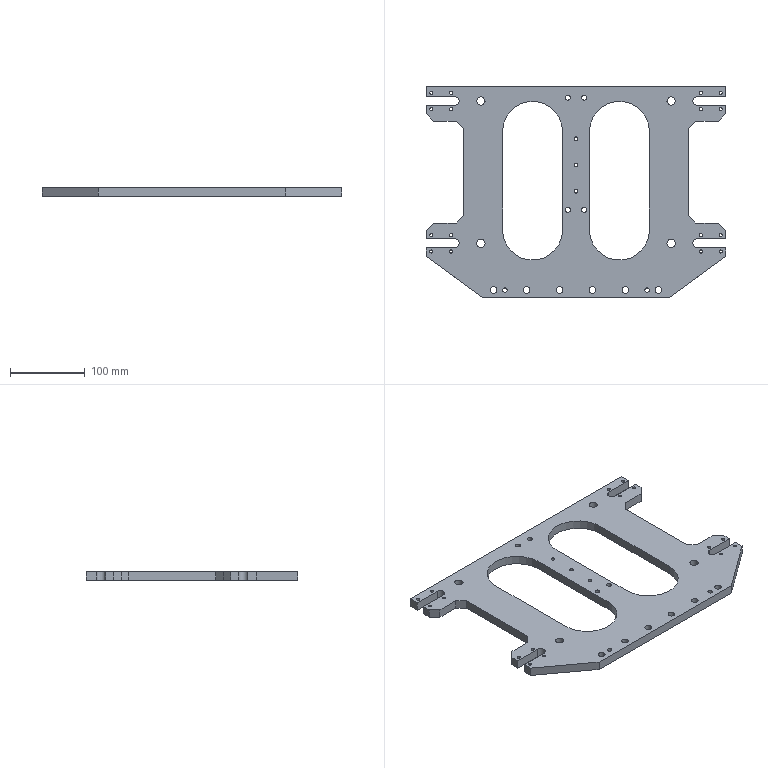CAM job | NX | 3-axis milling, drilling | part box 400 x 282 x 12 mm | stock box 404 x 286 x 12 mm
Tools:
number,name,description,diameter,corner_radius,flute_length,length,flutes
11,ZXZ,Milling Tool-5 Parameters,6.0,0.0,50.0,75.0,2
16,6.0ZT,Drilling Tool,6.0,0.0,35.0,50.0,2
15,5.0ZT,Drilling Tool,5.0,0.0,35.0,50.0,2
17,6.6ZT,Drilling Tool,6.6,0.0,35.0,50.0,2
14,4.2ZT,Drilling Tool,4.2,0.0,35.0,50.0,2
19,9.0ZT,Drilling Tool,9.0,0.0,35.0,50.0,2
12,11.0ZT,Drilling Tool,11.0,0.0,35.0,50.0,2
10,D10,Milling Tool-5 Parameters,10.0,0.0,50.0,75.0,2
9,D10JING,Milling Tool-5 Parameters,10.0,0.0,50.0,75.0,2
6,D6,Milling Tool-5 Parameters,6.0,0.0,50.0,75.0,2
7,D6A45,Milling Tool-5 Parameters,6.0,0.0,3.0,3.0,2
Operations:
program,operation,operation_type,tool,method,geometry_group,spindle_rpm,surface_speed,feed_per_tooth,feed_cut,feed_plunge,cut_length_mm,path_length_mm,cut_time_min,machine_time_min
1压左右,DRILLING,Operation,ZXZ,METHOD,A,3000.0,56.0,0.0417,250.0,0.0,140.0,1965.674,0.56,0.7426
1压左右,DRILLING_COPY,Operation,6.0ZT,METHOD,A,2000.0,37.0,0.045,180.0,0.0,36.605,426.234,0.2034,0.2423
1压左右,DRILLING_COPY_COPY_3,Operation,5.0ZT,METHOD,A,2000.0,37.0,0.045,180.0,0.0,54.007,344.27,0.3,0.3291
1压左右,DRILLING_COPY_COPY_2,Operation,6.6ZT,METHOD,A,2000.0,37.0,0.045,180.0,0.0,73.931,510.904,0.4107,0.4544
1压左右,DRILLING_COPY_COPY_1,Operation,4.2ZT,METHOD,A,2000.0,37.0,0.045,180.0,0.0,284.189,1727.548,1.579,1.723
1压左右,DRILLING_COPY_COPY,Operation,9.0ZT,METHOD,A,1000.0,28.0,0.09,180.0,0.0,115.223,625.957,0.6401,0.6912
1压左右,DRILLING_COPY_COPY_COPY,Operation,11.0ZT,METHOD,A,1000.0,28.0,0.09,180.0,0.0,79.219,1024.7,0.4401,0.5347
1压左右,ZLEVEL_PROFILE,ZLevelMilling,D10,METHOD,A,2200.0,69.0,0.5,2200.0,100.0,49399.267,49994.898,22.454,22.514
1压左右,ZLEVEL_PROFILE_COPY_1,ZLevelMilling,D10,METHOD,A,2200.0,69.0,0.5,2200.0,100.0,52254.708,52716.969,23.752,23.798
1压左右,ZLEVEL_PROFILE_COPY,ZLevelMilling,D10JING,METHOD,A,5000.0,157.0,0.12,1200.0,100.0,876.934,1475.247,0.7308,0.7906
1压左右,ZLEVEL_PROFILE_COPY_COPY_1,ZLevelMilling,D6,METHOD,A,5000.0,157.0,0.12,1200.0,100.0,1006.043,1592.897,0.8384,0.8971
1压左右,ZLEVEL_PROFILE_COPY_COPY,ZLevelMilling,D6A45,METHOD,A,7500.0,141.0,0.08,1200.0,100.0,2681.248,14655.066,2.234,3.432
2压前后,ZLEVEL_PROFILE_COPY_1_1,ZLevelMilling,D10,METHOD,A,2200.0,69.0,0.5,2200.0,100.0,54566.202,55341.754,24.803,24.88
2压前后,ZLEVEL_PROFILE_COPY_COPY_1_1,ZLevelMilling,D10JING,METHOD,A,5000.0,157.0,0.12,1200.0,100.0,971.41,1746.381,0.8095,0.887
2压前后,ZLEVEL_PROFILE_COPY_COPY_COPY,ZLevelMilling,D6A45,METHOD,A,7500.0,141.0,0.08,1200.0,100.0,962.652,1678.48,0.8022,0.8738